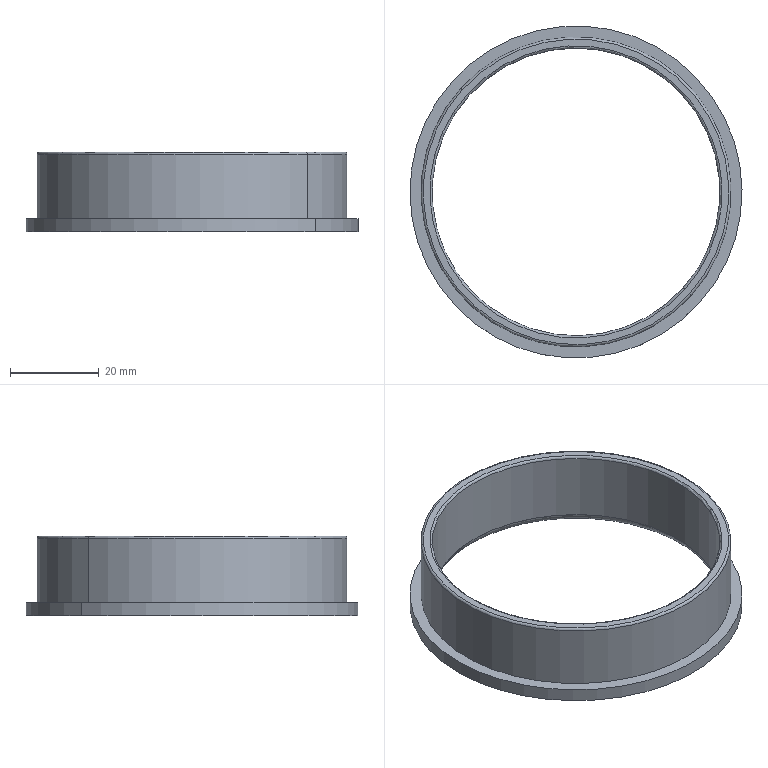Part | NX | features solid 2 | 1 solid | 15 faces | box 75 x 75 x 18 mm | volume 11050 mm3 | torus 6 | cylinder 6 | plane 3 | commonest cylinder face diameters 65 x2 70 x2 75 x2
STEP:
#1=CARTESIAN_POINT('',(-475.678,-1611.959,980.));
#2=VERTEX_POINT('',#1);
#3=CARTESIAN_POINT('',(-476.05,-1611.625,979.5));
#4=VERTEX_POINT('',#3);
#5=CARTESIAN_POINT('',(-475.678,-1611.959,979.5));
#6=DIRECTION('',(0.6679,0.7443,0.));
#7=DIRECTION('',(-0.7443,0.6679,0.));
#8=AXIS2_PLACEMENT_3D('',#5,#6,#7);
#9=CIRCLE('',#8,0.5);
#10=EDGE_CURVE('',#2,#4,#9,.F.);
#11=ORIENTED_EDGE('',*,*,#10,.T.);
#12=CARTESIAN_POINT('',(-423.95,-1658.375,979.5));
#13=VERTEX_POINT('',#12);
#14=CARTESIAN_POINT('',(-450.,-1635.,979.5));
#15=DIRECTION('',(0.,0.,-1.));
#16=DIRECTION('',(0.7443,-0.6679,0.));
#17=AXIS2_PLACEMENT_3D('',#14,#15,#16);
#18=CIRCLE('',#17,35.);
#19=EDGE_CURVE('',#13,#4,#18,.T.);
#20=ORIENTED_EDGE('',*,*,#19,.F.);
#21=CARTESIAN_POINT('',(-424.322,-1658.041,980.));
#22=VERTEX_POINT('',#21);
#23=CARTESIAN_POINT('',(-424.322,-1658.041,979.5));
#24=DIRECTION('',(-0.6679,-0.7443,0.));
#25=DIRECTION('',(0.7443,-0.6679,0.));
#26=AXIS2_PLACEMENT_3D('',#23,#24,#25);
#27=CIRCLE('',#26,0.5);
#28=EDGE_CURVE('',#13,#22,#27,.T.);
#29=ORIENTED_EDGE('',*,*,#28,.T.);
#30=CARTESIAN_POINT('',(-450.,-1635.,980.));
#31=DIRECTION('',(0.,0.,1.));
#32=DIRECTION('',(0.7443,-0.6679,0.));
#33=AXIS2_PLACEMENT_3D('',#30,#31,#32);
#34=CIRCLE('',#33,34.5);
#35=EDGE_CURVE('',#2,#22,#34,.T.);
#36=ORIENTED_EDGE('',*,*,#35,.F.);
#37=EDGE_LOOP('',(#11,#20,#29,#36));
#38=FACE_BOUND('',#37,.T.);
#39=CARTESIAN_POINT('',(-450.,-1635.,979.5));
#40=DIRECTION('',(0.,0.,1.));
#41=DIRECTION('',(0.7443,-0.6679,0.));
#42=AXIS2_PLACEMENT_3D('',#39,#40,#41);
#43=TOROIDAL_SURFACE('',#42,34.5,0.5);
#44=ADVANCED_FACE('',(#38),#43,.T.);
#45=CARTESIAN_POINT('',(-474.189,-1613.294,979.5));
#46=VERTEX_POINT('',#45);
#47=CARTESIAN_POINT('',(-474.561,-1612.96,980.));
#48=VERTEX_POINT('',#47);
#49=CARTESIAN_POINT('',(-474.561,-1612.96,979.5));
#50=DIRECTION('',(0.6679,0.7443,0.));
#51=DIRECTION('',(-0.7443,0.6679,0.));
#52=AXIS2_PLACEMENT_3D('',#49,#50,#51);
#53=CIRCLE('',#52,0.5);
#54=EDGE_CURVE('',#46,#48,#53,.F.);
#55=ORIENTED_EDGE('',*,*,#54,.T.);
#56=CARTESIAN_POINT('',(-425.439,-1657.04,980.));
#57=VERTEX_POINT('',#56);
#58=CARTESIAN_POINT('',(-450.,-1635.,980.));
#59=DIRECTION('',(0.,0.,-1.));
#60=DIRECTION('',(0.7443,-0.6679,0.));
#61=AXIS2_PLACEMENT_3D('',#58,#59,#60);
#62=CIRCLE('',#61,33.);
#63=EDGE_CURVE('',#57,#48,#62,.T.);
#64=ORIENTED_EDGE('',*,*,#63,.F.);
#65=CARTESIAN_POINT('',(-425.811,-1656.706,979.5));
#66=VERTEX_POINT('',#65);
#67=CARTESIAN_POINT('',(-425.439,-1657.04,979.5));
#68=DIRECTION('',(-0.6679,-0.7443,0.));
#69=DIRECTION('',(0.7443,-0.6679,0.));
#70=AXIS2_PLACEMENT_3D('',#67,#68,#69);
#71=CIRCLE('',#70,0.5);
#72=EDGE_CURVE('',#57,#66,#71,.T.);
#73=ORIENTED_EDGE('',*,*,#72,.T.);
#74=CARTESIAN_POINT('',(-450.,-1635.,979.5));
#75=DIRECTION('',(0.,0.,1.));
#76=DIRECTION('',(0.7443,-0.6679,0.));
#77=AXIS2_PLACEMENT_3D('',#74,#75,#76);
#78=CIRCLE('',#77,32.5);
#79=EDGE_CURVE('',#46,#66,#78,.T.);
#80=ORIENTED_EDGE('',*,*,#79,.F.);
#81=EDGE_LOOP('',(#55,#64,#73,#80));
#82=FACE_BOUND('',#81,.T.);
#83=CARTESIAN_POINT('',(-450.,-1635.,979.5));
#84=DIRECTION('',(0.,0.,1.));
#85=DIRECTION('',(0.7443,-0.6679,0.));
#86=AXIS2_PLACEMENT_3D('',#83,#84,#85);
#87=TOROIDAL_SURFACE('',#86,33.,0.5);
#88=ADVANCED_FACE('',(#82),#87,.T.);
#89=CARTESIAN_POINT('',(-424.322,-1658.041,962.));
#90=VERTEX_POINT('',#89);
#91=CARTESIAN_POINT('',(-425.811,-1656.706,964.));
#92=VERTEX_POINT('',#91);
#93=CARTESIAN_POINT('',(-424.322,-1658.041,964.));
#94=DIRECTION('',(0.6679,0.7443,0.));
#95=DIRECTION('',(-0.7443,0.6679,0.));
#96=AXIS2_PLACEMENT_3D('',#93,#94,#95);
#97=CIRCLE('',#96,2.);
#98=EDGE_CURVE('',#90,#92,#97,.T.);
#99=ORIENTED_EDGE('',*,*,#98,.F.);
#100=CARTESIAN_POINT('',(-475.678,-1611.959,962.));
#101=VERTEX_POINT('',#100);
#102=CARTESIAN_POINT('',(-450.,-1635.,962.));
#103=DIRECTION('',(0.,0.,1.));
#104=DIRECTION('',(-0.7443,0.6679,0.));
#105=AXIS2_PLACEMENT_3D('',#102,#103,#104);
#106=CIRCLE('',#105,34.5);
#107=EDGE_CURVE('',#101,#90,#106,.T.);
#108=ORIENTED_EDGE('',*,*,#107,.F.);
#109=CARTESIAN_POINT('',(-474.189,-1613.294,964.));
#110=VERTEX_POINT('',#109);
#111=CARTESIAN_POINT('',(-475.678,-1611.959,964.));
#112=DIRECTION('',(-0.6679,-0.7443,0.));
#113=DIRECTION('',(0.7443,-0.6679,0.));
#114=AXIS2_PLACEMENT_3D('',#111,#112,#113);
#115=CIRCLE('',#114,2.);
#116=EDGE_CURVE('',#110,#101,#115,.F.);
#117=ORIENTED_EDGE('',*,*,#116,.F.);
#118=CARTESIAN_POINT('',(-450.,-1635.,964.));
#119=DIRECTION('',(0.,0.,-1.));
#120=DIRECTION('',(-0.7443,0.6679,0.));
#121=AXIS2_PLACEMENT_3D('',#118,#119,#120);
#122=CIRCLE('',#121,32.5);
#123=EDGE_CURVE('',#92,#110,#122,.T.);
#124=ORIENTED_EDGE('',*,*,#123,.F.);
#125=EDGE_LOOP('',(#99,#108,#117,#124));
#126=FACE_BOUND('',#125,.T.);
#127=CARTESIAN_POINT('',(-450.,-1635.,964.));
#128=DIRECTION('',(0.,0.,-1.));
#129=DIRECTION('',(-0.7443,0.6679,0.));
#130=AXIS2_PLACEMENT_3D('',#127,#128,#129);
#131=TOROIDAL_SURFACE('',#130,34.5,2.);
#132=ADVANCED_FACE('',(#126),#131,.T.);
#133=CARTESIAN_POINT('',(-423.95,-1658.375,965.));
#134=VERTEX_POINT('',#133);
#135=CARTESIAN_POINT('',(-423.95,-1658.375,1016.));
#136=DIRECTION('',(0.,0.,-1.));
#137=VECTOR('',#136,1000.);
#138=LINE('',#135,#137);
#139=EDGE_CURVE('',#13,#134,#138,.T.);
#140=ORIENTED_EDGE('',*,*,#139,.F.);
#141=ORIENTED_EDGE('',*,*,#19,.T.);
#142=CARTESIAN_POINT('',(-476.05,-1611.625,965.));
#143=VERTEX_POINT('',#142);
#144=CARTESIAN_POINT('',(-476.05,-1611.625,1016.));
#145=DIRECTION('',(0.,0.,-1.));
#146=VECTOR('',#145,1000.);
#147=LINE('',#144,#146);
#148=EDGE_CURVE('',#143,#4,#147,.F.);
#149=ORIENTED_EDGE('',*,*,#148,.F.);
#150=CARTESIAN_POINT('',(-450.,-1635.,965.));
#151=DIRECTION('',(0.,0.,-1.));
#152=DIRECTION('',(-0.7443,0.6679,0.));
#153=AXIS2_PLACEMENT_3D('',#150,#151,#152);
#154=CIRCLE('',#153,35.);
#155=EDGE_CURVE('',#134,#143,#154,.T.);
#156=ORIENTED_EDGE('',*,*,#155,.F.);
#157=EDGE_LOOP('',(#140,#141,#149,#156));
#158=FACE_BOUND('',#157,.T.);
#159=CARTESIAN_POINT('',(-450.,-1635.,1016.));
#160=DIRECTION('',(0.,0.,-1.));
#161=DIRECTION('',(-0.7443,0.6679,0.));
#162=AXIS2_PLACEMENT_3D('',#159,#160,#161);
#163=CYLINDRICAL_SURFACE('',#162,35.);
#164=ADVANCED_FACE('',(#158),#163,.T.);
#165=CARTESIAN_POINT('',(-450.,-1635.,965.));
#166=DIRECTION('',(0.,0.,-1.));
#167=DIRECTION('',(-0.7443,0.6679,0.));
#168=AXIS2_PLACEMENT_3D('',#165,#166,#167);
#169=CIRCLE('',#168,35.);
#170=EDGE_CURVE('',#143,#134,#169,.T.);
#171=ORIENTED_EDGE('',*,*,#170,.T.);
#172=ORIENTED_EDGE('',*,*,#155,.T.);
#173=EDGE_LOOP('',(#171,#172));
#174=FACE_BOUND('',#173,.T.);
#175=CARTESIAN_POINT('',(-477.91,-1609.955,965.));
#176=VERTEX_POINT('',#175);
#177=CARTESIAN_POINT('',(-422.09,-1660.045,965.));
#178=VERTEX_POINT('',#177);
#179=CARTESIAN_POINT('',(-450.,-1635.,965.));
#180=DIRECTION('',(0.,0.,-1.));
#181=DIRECTION('',(-0.7443,0.6679,0.));
#182=AXIS2_PLACEMENT_3D('',#179,#180,#181);
#183=CIRCLE('',#182,37.5);
#184=EDGE_CURVE('',#176,#178,#183,.T.);
#185=ORIENTED_EDGE('',*,*,#184,.F.);
#186=CARTESIAN_POINT('',(-450.,-1635.,965.));
#187=DIRECTION('',(0.,0.,-1.));
#188=DIRECTION('',(-0.7443,0.6679,0.));
#189=AXIS2_PLACEMENT_3D('',#186,#187,#188);
#190=CIRCLE('',#189,37.5);
#191=EDGE_CURVE('',#178,#176,#190,.T.);
#192=ORIENTED_EDGE('',*,*,#191,.F.);
#193=EDGE_LOOP('',(#185,#192));
#194=FACE_BOUND('',#193,.T.);
#195=CARTESIAN_POINT('',(-477.91,-1609.955,965.));
#196=DIRECTION('',(0.,0.,1.));
#197=DIRECTION('',(0.,-1.,0.));
#198=AXIS2_PLACEMENT_3D('',#195,#196,#197);
#199=PLANE('',#198);
#200=ADVANCED_FACE('',(#174,#194),#199,.T.);
#201=CARTESIAN_POINT('',(-422.09,-1660.045,962.));
#202=VERTEX_POINT('',#201);
#203=CARTESIAN_POINT('',(-422.09,-1660.045,1016.));
#204=DIRECTION('',(0.,0.,-1.));
#205=VECTOR('',#204,1000.);
#206=LINE('',#203,#205);
#207=EDGE_CURVE('',#202,#178,#206,.F.);
#208=ORIENTED_EDGE('',*,*,#207,.T.);
#209=ORIENTED_EDGE('',*,*,#191,.T.);
#210=CARTESIAN_POINT('',(-477.91,-1609.955,962.));
#211=VERTEX_POINT('',#210);
#212=CARTESIAN_POINT('',(-477.91,-1609.955,1016.));
#213=DIRECTION('',(0.,0.,-1.));
#214=VECTOR('',#213,1000.);
#215=LINE('',#212,#214);
#216=EDGE_CURVE('',#176,#211,#215,.T.);
#217=ORIENTED_EDGE('',*,*,#216,.T.);
#218=CARTESIAN_POINT('',(-450.,-1635.,962.));
#219=DIRECTION('',(0.,0.,-1.));
#220=DIRECTION('',(-0.7443,0.6679,0.));
#221=AXIS2_PLACEMENT_3D('',#218,#219,#220);
#222=CIRCLE('',#221,37.5);
#223=EDGE_CURVE('',#202,#211,#222,.T.);
#224=ORIENTED_EDGE('',*,*,#223,.F.);
#225=EDGE_LOOP('',(#208,#209,#217,#224));
#226=FACE_BOUND('',#225,.T.);
#227=CARTESIAN_POINT('',(-450.,-1635.,1016.));
#228=DIRECTION('',(0.,0.,-1.));
#229=DIRECTION('',(-0.7443,0.6679,0.));
#230=AXIS2_PLACEMENT_3D('',#227,#228,#229);
#231=CYLINDRICAL_SURFACE('',#230,37.5);
#232=ADVANCED_FACE('',(#226),#231,.T.);
#233=ORIENTED_EDGE('',*,*,#107,.T.);
#234=CARTESIAN_POINT('',(-450.,-1635.,962.));
#235=DIRECTION('',(0.,0.,1.));
#236=DIRECTION('',(-0.7443,0.6679,0.));
#237=AXIS2_PLACEMENT_3D('',#234,#235,#236);
#238=CIRCLE('',#237,34.5);
#239=EDGE_CURVE('',#90,#101,#238,.T.);
#240=ORIENTED_EDGE('',*,*,#239,.T.);
#241=EDGE_LOOP('',(#233,#240));
#242=FACE_BOUND('',#241,.T.);
#243=CARTESIAN_POINT('',(-450.,-1635.,962.));
#244=DIRECTION('',(0.,0.,-1.));
#245=DIRECTION('',(-0.7443,0.6679,0.));
#246=AXIS2_PLACEMENT_3D('',#243,#244,#245);
#247=CIRCLE('',#246,37.5);
#248=EDGE_CURVE('',#211,#202,#247,.T.);
#249=ORIENTED_EDGE('',*,*,#248,.T.);
#250=ORIENTED_EDGE('',*,*,#223,.T.);
#251=EDGE_LOOP('',(#249,#250));
#252=FACE_BOUND('',#251,.T.);
#253=CARTESIAN_POINT('',(-474.189,-1613.294,962.));
#254=DIRECTION('',(0.,0.,-1.));
#255=DIRECTION('',(0.,-1.,0.));
#256=AXIS2_PLACEMENT_3D('',#253,#254,#255);
#257=PLANE('',#256);
#258=ADVANCED_FACE('',(#242,#252),#257,.T.);
#259=CARTESIAN_POINT('',(-425.811,-1656.706,1016.));
#260=DIRECTION('',(0.,0.,-1.));
#261=VECTOR('',#260,1000.);
#262=LINE('',#259,#261);
#263=EDGE_CURVE('',#92,#66,#262,.F.);
#264=ORIENTED_EDGE('',*,*,#263,.T.);
#265=CARTESIAN_POINT('',(-450.,-1635.,979.5));
#266=DIRECTION('',(0.,0.,1.));
#267=DIRECTION('',(0.7443,-0.6679,0.));
#268=AXIS2_PLACEMENT_3D('',#265,#266,#267);
#269=CIRCLE('',#268,32.5);
#270=EDGE_CURVE('',#66,#46,#269,.T.);
#271=ORIENTED_EDGE('',*,*,#270,.T.);
#272=CARTESIAN_POINT('',(-474.189,-1613.294,1016.));
#273=DIRECTION('',(0.,0.,-1.));
#274=VECTOR('',#273,1000.);
#275=LINE('',#272,#274);
#276=EDGE_CURVE('',#46,#110,#275,.T.);
#277=ORIENTED_EDGE('',*,*,#276,.T.);
#278=CARTESIAN_POINT('',(-450.,-1635.,964.));
#279=DIRECTION('',(0.,0.,-1.));
#280=DIRECTION('',(-0.7443,0.6679,0.));
#281=AXIS2_PLACEMENT_3D('',#278,#279,#280);
#282=CIRCLE('',#281,32.5);
#283=EDGE_CURVE('',#110,#92,#282,.T.);
#284=ORIENTED_EDGE('',*,*,#283,.T.);
#285=EDGE_LOOP('',(#264,#271,#277,#284));
#286=FACE_BOUND('',#285,.T.);
#287=CARTESIAN_POINT('',(-450.,-1635.,1016.));
#288=DIRECTION('',(0.,0.,-1.));
#289=DIRECTION('',(-0.7443,0.6679,0.));
#290=AXIS2_PLACEMENT_3D('',#287,#288,#289);
#291=CYLINDRICAL_SURFACE('',#290,32.5);
#292=ADVANCED_FACE('',(#286),#291,.F.);
#293=ORIENTED_EDGE('',*,*,#63,.T.);
#294=CARTESIAN_POINT('',(-450.,-1635.,980.));
#295=DIRECTION('',(0.,0.,-1.));
#296=DIRECTION('',(0.7443,-0.6679,0.));
#297=AXIS2_PLACEMENT_3D('',#294,#295,#296);
#298=CIRCLE('',#297,33.);
#299=EDGE_CURVE('',#48,#57,#298,.T.);
#300=ORIENTED_EDGE('',*,*,#299,.T.);
#301=EDGE_LOOP('',(#293,#300));
#302=FACE_BOUND('',#301,.T.);
#303=CARTESIAN_POINT('',(-450.,-1635.,980.));
#304=DIRECTION('',(0.,0.,1.));
#305=DIRECTION('',(0.7443,-0.6679,0.));
#306=AXIS2_PLACEMENT_3D('',#303,#304,#305);
#307=CIRCLE('',#306,34.5);
#308=EDGE_CURVE('',#22,#2,#307,.T.);
#309=ORIENTED_EDGE('',*,*,#308,.T.);
#310=ORIENTED_EDGE('',*,*,#35,.T.);
#311=EDGE_LOOP('',(#309,#310));
#312=FACE_BOUND('',#311,.T.);
#313=CARTESIAN_POINT('',(-476.05,-1611.625,980.));
#314=DIRECTION('',(0.,0.,1.));
#315=DIRECTION('',(0.,-1.,0.));
#316=AXIS2_PLACEMENT_3D('',#313,#314,#315);
#317=PLANE('',#316);
#318=ADVANCED_FACE('',(#302,#312),#317,.T.);
#319=ORIENTED_EDGE('',*,*,#79,.T.);
#320=ORIENTED_EDGE('',*,*,#263,.F.);
#321=ORIENTED_EDGE('',*,*,#123,.T.);
#322=ORIENTED_EDGE('',*,*,#276,.F.);
#323=EDGE_LOOP('',(#319,#320,#321,#322));
#324=FACE_BOUND('',#323,.T.);
#325=CARTESIAN_POINT('',(-450.,-1635.,1016.));
#326=DIRECTION('',(0.,0.,-1.));
#327=DIRECTION('',(-0.7443,0.6679,0.));
#328=AXIS2_PLACEMENT_3D('',#325,#326,#327);
#329=CYLINDRICAL_SURFACE('',#328,32.5);
#330=ADVANCED_FACE('',(#324),#329,.F.);
#331=ORIENTED_EDGE('',*,*,#184,.T.);
#332=ORIENTED_EDGE('',*,*,#207,.F.);
#333=ORIENTED_EDGE('',*,*,#248,.F.);
#334=ORIENTED_EDGE('',*,*,#216,.F.);
#335=EDGE_LOOP('',(#331,#332,#333,#334));
#336=FACE_BOUND('',#335,.T.);
#337=CARTESIAN_POINT('',(-450.,-1635.,1016.));
#338=DIRECTION('',(0.,0.,-1.));
#339=DIRECTION('',(-0.7443,0.6679,0.));
#340=AXIS2_PLACEMENT_3D('',#337,#338,#339);
#341=CYLINDRICAL_SURFACE('',#340,37.5);
#342=ADVANCED_FACE('',(#336),#341,.T.);
#343=CARTESIAN_POINT('',(-450.,-1635.,979.5));
#344=DIRECTION('',(0.,0.,-1.));
#345=DIRECTION('',(0.7443,-0.6679,0.));
#346=AXIS2_PLACEMENT_3D('',#343,#344,#345);
#347=CIRCLE('',#346,35.);
#348=EDGE_CURVE('',#4,#13,#347,.T.);
#349=ORIENTED_EDGE('',*,*,#348,.T.);
#350=ORIENTED_EDGE('',*,*,#139,.T.);
#351=ORIENTED_EDGE('',*,*,#170,.F.);
#352=ORIENTED_EDGE('',*,*,#148,.T.);
#353=EDGE_LOOP('',(#349,#350,#351,#352));
#354=FACE_BOUND('',#353,.T.);
#355=CARTESIAN_POINT('',(-450.,-1635.,1016.));
#356=DIRECTION('',(0.,0.,-1.));
#357=DIRECTION('',(-0.7443,0.6679,0.));
#358=AXIS2_PLACEMENT_3D('',#355,#356,#357);
#359=CYLINDRICAL_SURFACE('',#358,35.);
#360=ADVANCED_FACE('',(#354),#359,.T.);
#361=ORIENTED_EDGE('',*,*,#239,.F.);
#362=ORIENTED_EDGE('',*,*,#98,.T.);
#363=ORIENTED_EDGE('',*,*,#283,.F.);
#364=ORIENTED_EDGE('',*,*,#116,.T.);
#365=EDGE_LOOP('',(#361,#362,#363,#364));
#366=FACE_BOUND('',#365,.T.);
#367=CARTESIAN_POINT('',(-450.,-1635.,964.));
#368=DIRECTION('',(0.,0.,-1.));
#369=DIRECTION('',(-0.7443,0.6679,0.));
#370=AXIS2_PLACEMENT_3D('',#367,#368,#369);
#371=TOROIDAL_SURFACE('',#370,34.5,2.);
#372=ADVANCED_FACE('',(#366),#371,.T.);
#373=ORIENTED_EDGE('',*,*,#299,.F.);
#374=ORIENTED_EDGE('',*,*,#54,.F.);
#375=ORIENTED_EDGE('',*,*,#270,.F.);
#376=ORIENTED_EDGE('',*,*,#72,.F.);
#377=EDGE_LOOP('',(#373,#374,#375,#376));
#378=FACE_BOUND('',#377,.T.);
#379=CARTESIAN_POINT('',(-450.,-1635.,979.5));
#380=DIRECTION('',(0.,0.,1.));
#381=DIRECTION('',(0.7443,-0.6679,0.));
#382=AXIS2_PLACEMENT_3D('',#379,#380,#381);
#383=TOROIDAL_SURFACE('',#382,33.,0.5);
#384=ADVANCED_FACE('',(#378),#383,.T.);
#385=ORIENTED_EDGE('',*,*,#348,.F.);
#386=ORIENTED_EDGE('',*,*,#10,.F.);
#387=ORIENTED_EDGE('',*,*,#308,.F.);
#388=ORIENTED_EDGE('',*,*,#28,.F.);
#389=EDGE_LOOP('',(#385,#386,#387,#388));
#390=FACE_BOUND('',#389,.T.);
#391=CARTESIAN_POINT('',(-450.,-1635.,979.5));
#392=DIRECTION('',(0.,0.,1.));
#393=DIRECTION('',(0.7443,-0.6679,0.));
#394=AXIS2_PLACEMENT_3D('',#391,#392,#393);
#395=TOROIDAL_SURFACE('',#394,34.5,0.5);
#396=ADVANCED_FACE('',(#390),#395,.T.);
#397=CLOSED_SHELL('',(#44,#88,#132,#164,#200,#232,#258,#292,#318,#330,#342,#360,#372,#384,#396));
#398=MANIFOLD_SOLID_BREP('',#397);
#399=(LENGTH_UNIT()NAMED_UNIT(*)SI_UNIT(.MILLI.,.METRE.));
#400=UNCERTAINTY_MEASURE_WITH_UNIT(LENGTH_MEASURE(0.00001),#399,'','');
#401=(NAMED_UNIT(*)PLANE_ANGLE_UNIT()SI_UNIT($,.RADIAN.));
#402=(NAMED_UNIT(*)SI_UNIT($,.STERADIAN.)SOLID_ANGLE_UNIT());
#403=(GEOMETRIC_REPRESENTATION_CONTEXT(3)GLOBAL_UNCERTAINTY_ASSIGNED_CONTEXT((#400))GLOBAL_UNIT_ASSIGNED_CONTEXT((#399,#401,#402))REPRESENTATION_CONTEXT('',''));
#404=ADVANCED_BREP_SHAPE_REPRESENTATION('',(#398),#403);